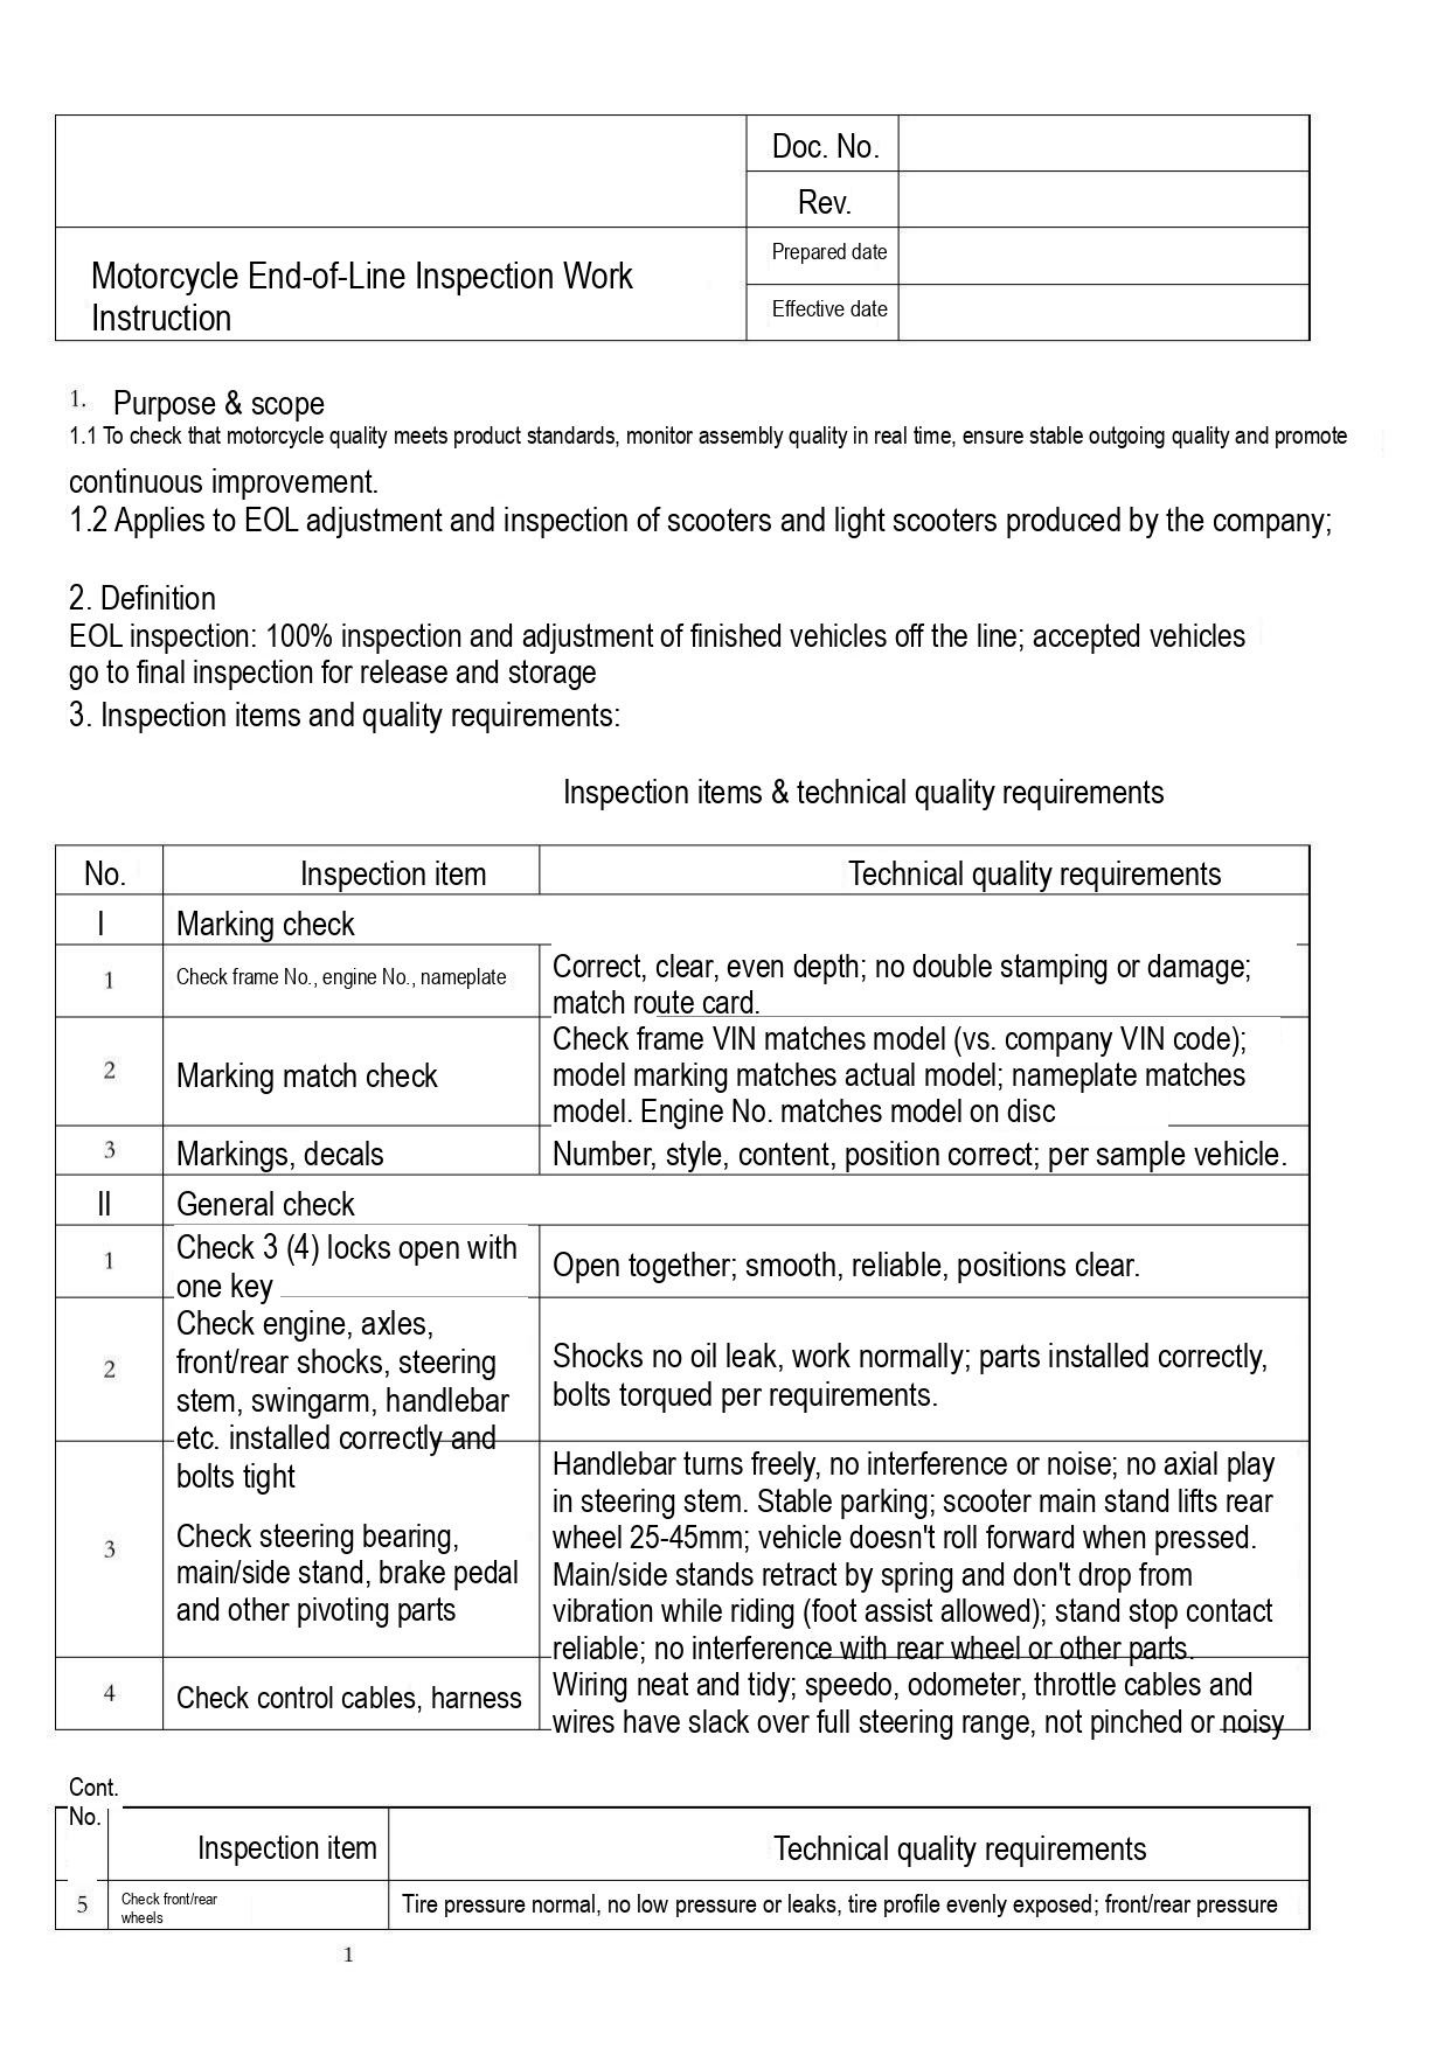| Motorcycle End-of-Line Inspection Work Instruction | Doc. No. | |
|---|---|---|
| | Rev. | |
| | Prepared date | |
| | Effective date | |

1. Purpose & scope
1.1 To check that motorcycle quality meets product standards, monitor assembly quality in real time, ensure stable outgoing quality and promote continuous improvement.
1.2 Applies to EOL adjustment and inspection of scooters and light scooters produced by the company;

2. Definition
EOL inspection: 100% inspection and adjustment of finished vehicles off the line; accepted vehicles go to final inspection for release and storage
3. Inspection items and quality requirements:

Inspection items & technical quality requirements

| No. | Inspection item | Technical quality requirements |
|---|---|---|
| I | Marking check | |
| 1 | Check frame No., engine No., nameplate | Correct, clear, even depth; no double stamping or damage; match route card. |
| 2 | Marking match check | Check frame VIN matches model (vs. company VIN code); model marking matches actual model; nameplate matches model. Engine No. matches model on disc |
| 3 | Markings, decals | Number, style, content, position correct; per sample vehicle. |
| II | General check | |
| 1 | Check 3 (4) locks open with one key | Open together; smooth, reliable, positions clear. |
| 2 | Check engine, axles, front/rear shocks, steering stem, swingarm, handlebar etc. installed correctly and bolts tight | Shocks no oil leak, work normally; parts installed correctly, bolts torqued per requirements. |
| 3 | Check steering bearing, main/side stand, brake pedal and other pivoting parts | Handlebar turns freely, no interference or noise; no axial play in steering stem. Stable parking; scooter main stand lifts rear wheel 25-45mm; vehicle doesn't roll forward when pressed. Main/side stands retract by spring and don't drop from vibration while riding (foot assist allowed); stand stop contact reliable; no interference with rear wheel or other parts. |
| 4 | Check control cables, harness | Wiring neat and tidy; speedo, odometer, throttle cables and wires have slack over full steering range, not pinched or noisy |

Cont.

| No. | Inspection item | Technical quality requirements |
|---|---|---|
| 5 | Check front/rear wheels | Tire pressure normal, no low pressure or leaks, tire profile evenly exposed; front/rear pressure |

1
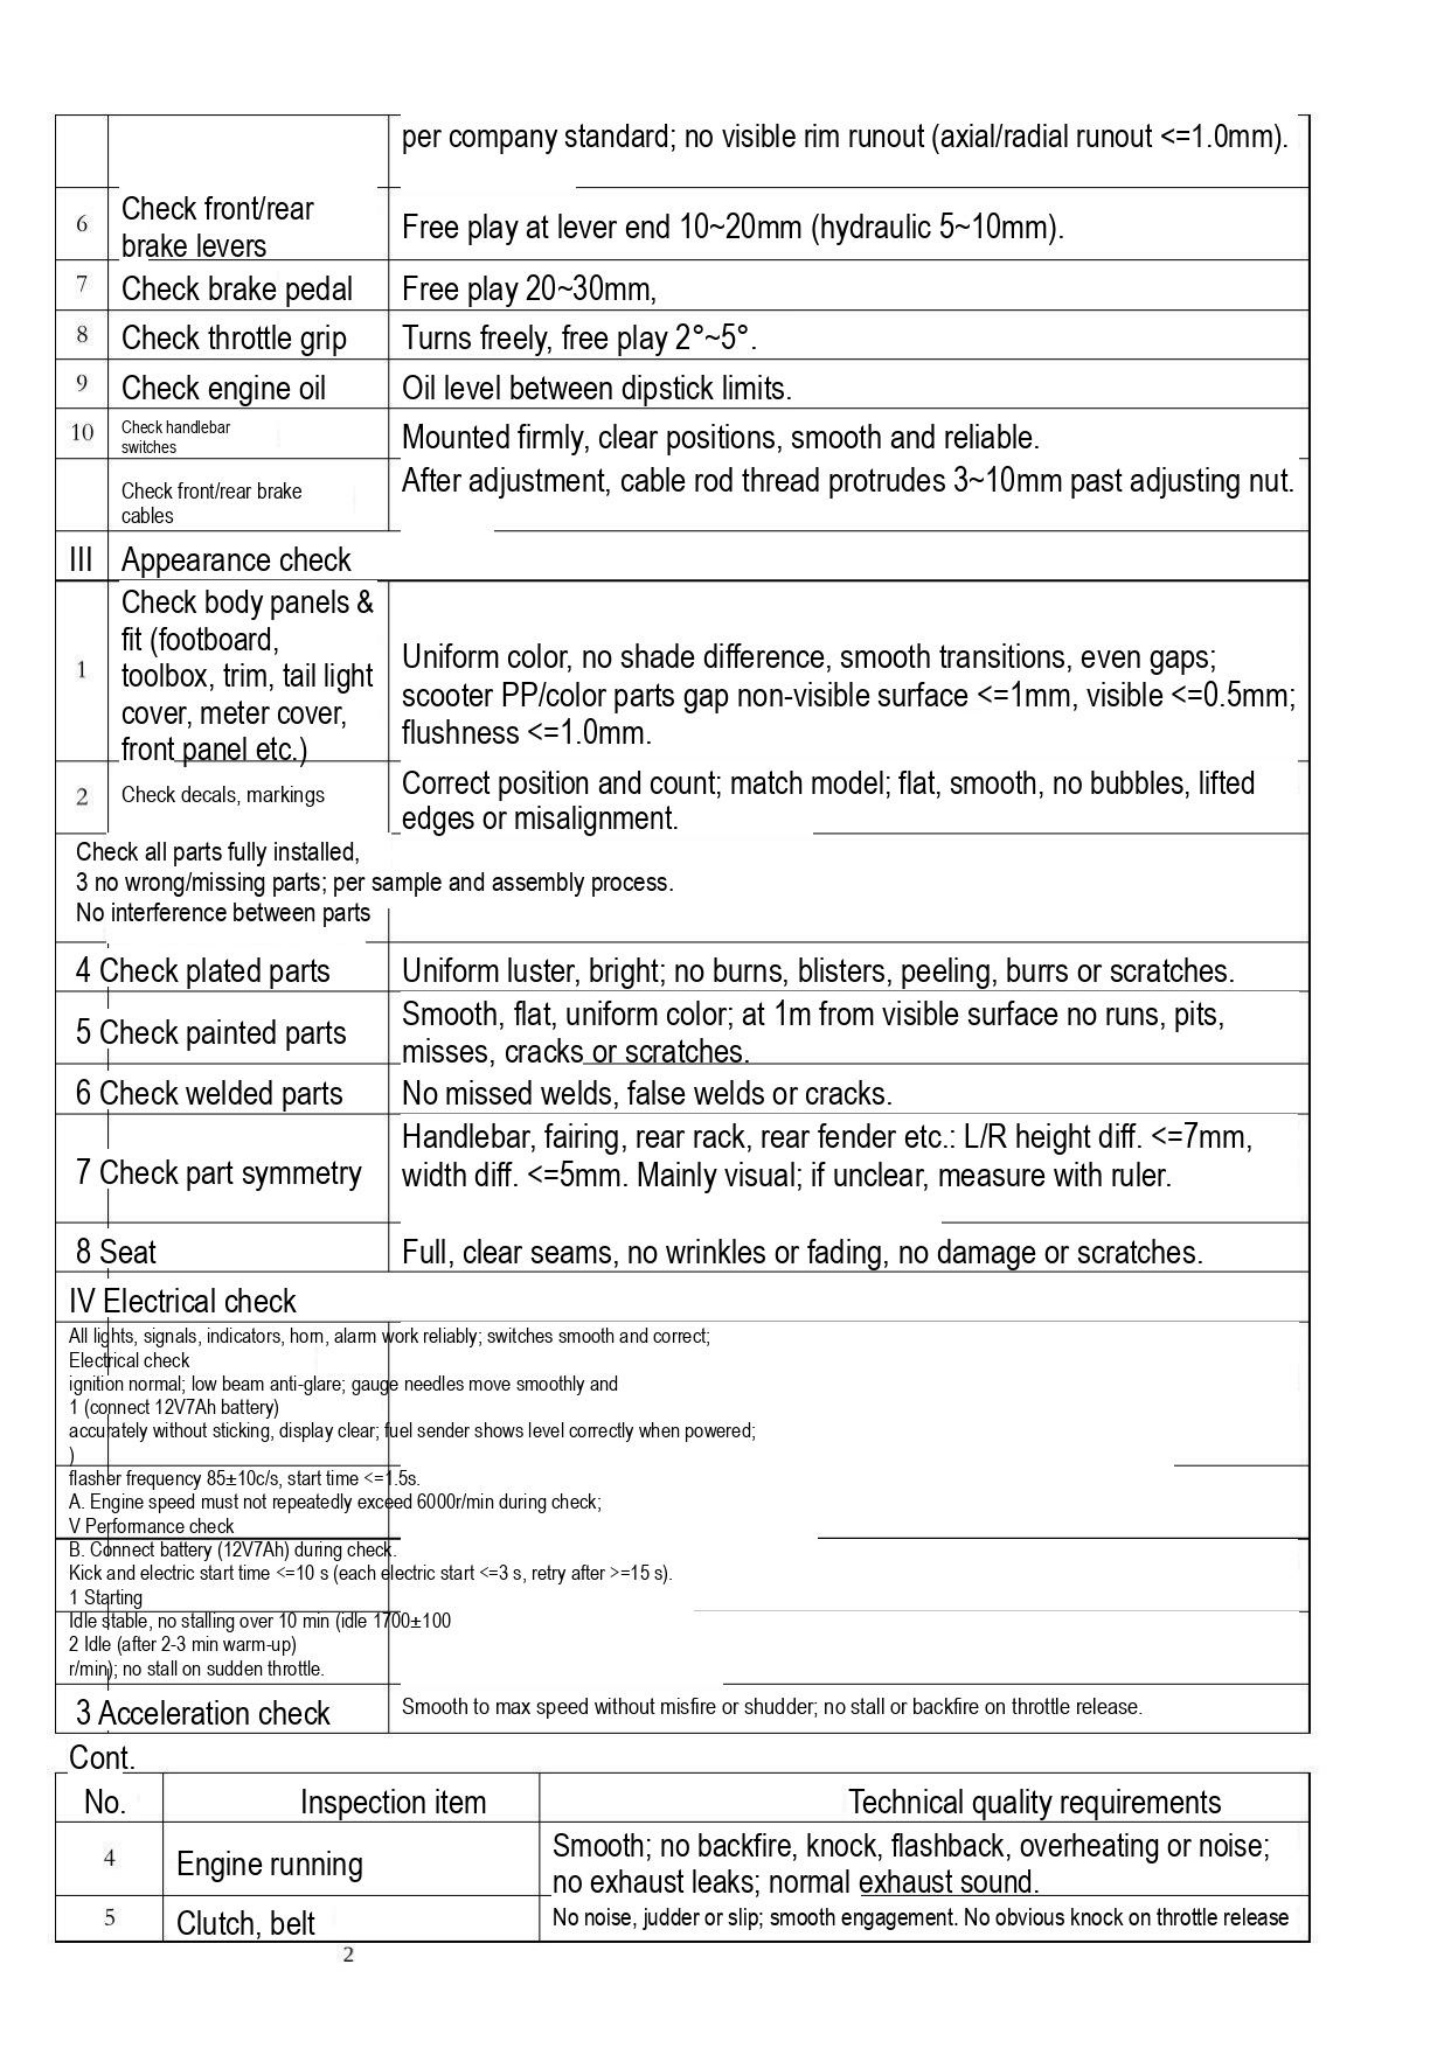| | | |
|---|---|---|
| | | per company standard; no visible rim runout (axial/radial runout <=1.0mm). |
| 6 | Check front/rear brake levers | Free play at lever end 10~20mm (hydraulic 5~10mm). |
| 7 | Check brake pedal | Free play 20~30mm, |
| 8 | Check throttle grip | Turns freely, free play 2°~5°. |
| 9 | Check engine oil | Oil level between dipstick limits. |
| 10 | Check handlebar switches | Mounted firmly, clear positions, smooth and reliable. |
| | Check front/rear brake cables | After adjustment, cable rod thread protrudes 3~10mm past adjusting nut. |
| III | Appearance check | |
| 1 | Check body panels & fit (footboard, toolbox, trim, tail light cover, meter cover, front panel etc.) | Uniform color, no shade difference, smooth transitions, even gaps; scooter PP/color parts gap non-visible surface <=1mm, visible <=0.5mm; flushness <=1.0mm. |
| 2 | Check decals, markings | Correct position and count; match model; flat, smooth, no bubbles, lifted edges or misalignment. |
| 3 | Check all parts fully installed, No interference between parts | no wrong/missing parts; per sample and assembly process. |
| 4 | Check plated parts | Uniform luster, bright; no burns, blisters, peeling, burrs or scratches. |
| 5 | Check painted parts | Smooth, flat, uniform color; at 1m from visible surface no runs, pits, misses, cracks or scratches. |
| 6 | Check welded parts | No missed welds, false welds or cracks. |
| 7 | Check part symmetry | Handlebar, fairing, rear rack, rear fender etc.: L/R height diff. <=7mm, width diff. <=5mm. Mainly visual; if unclear, measure with ruler. |
| 8 | Seat | Full, clear seams, no wrinkles or fading, no damage or scratches. |
| IV | Electrical check | |
| 1 | Electrical check (connect 12V7Ah battery) | All lights, signals, indicators, horn, alarm work reliably; switches smooth and correct; ignition normal; low beam anti-glare; gauge needles move smoothly and accurately without sticking, display clear; fuel sender shows level correctly when powered; flasher frequency 85±10c/s, start time <=1.5s. |
| V | Performance check | A. Engine speed must not repeatedly exceed 6000r/min during check; B. Connect battery (12V7Ah) during check. |
| 1 | Starting | Kick and electric start time <=10 s (each electric start <=3 s, retry after >=15 s). |
| 2 | Idle (after 2-3 min warm-up) | Idle stable, no stalling over 10 min (idle 1700±100 r/min); no stall on sudden throttle. |
| 3 | Acceleration check | Smooth to max speed without misfire or shudder; no stall or backfire on throttle release. |

Cont.

| No. | Inspection item | Technical quality requirements |
|---|---|---|
| 4 | Engine running | Smooth; no backfire, knock, flashback, overheating or noise; no exhaust leaks; normal exhaust sound. |
| 5 | Clutch, belt | No noise, judder or slip; smooth engagement. No obvious knock on throttle release |

2
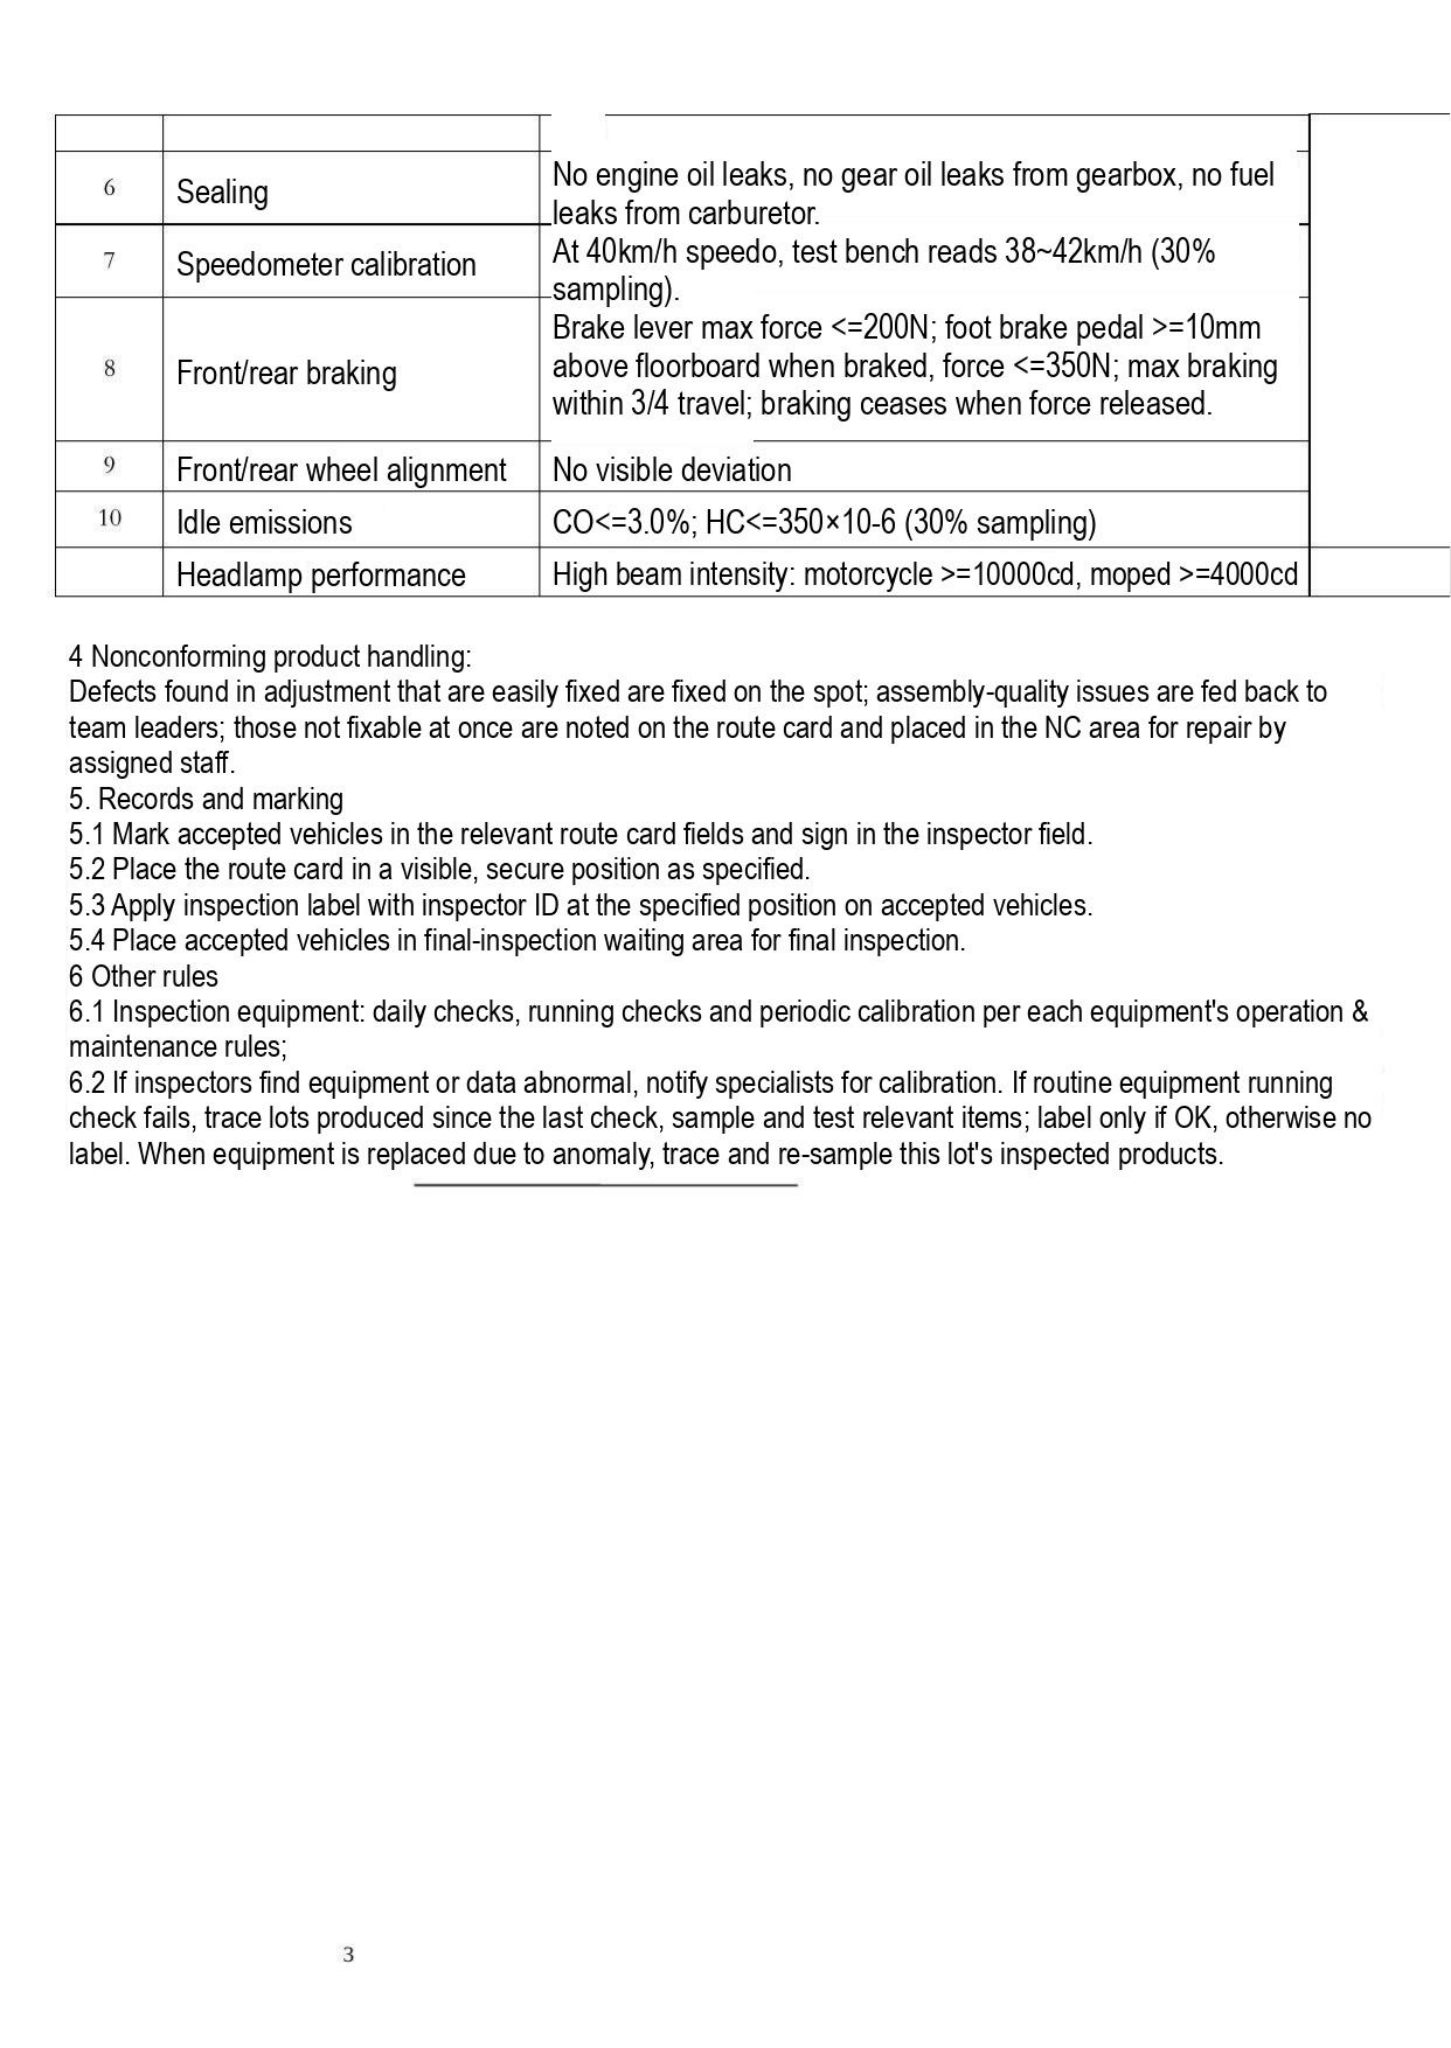| | | | |
|---|---|---|---|
| 6 | Sealing | No engine oil leaks, no gear oil leaks from gearbox, no fuel leaks from carburetor. | |
| 7 | Speedometer calibration | At 40km/h speedo, test bench reads 38~42km/h (30% sampling). | |
| 8 | Front/rear braking | Brake lever max force <=200N; foot brake pedal >=10mm above floorboard when braked, force <=350N; max braking within 3/4 travel; braking ceases when force released. | |
| 9 | Front/rear wheel alignment | No visible deviation | |
| 10 | Idle emissions | CO<=3.0%; HC<=350×10-6 (30% sampling) | |
| | Headlamp performance | High beam intensity: motorcycle >=10000cd, moped >=4000cd | |

4 Nonconforming product handling:
Defects found in adjustment that are easily fixed are fixed on the spot; assembly-quality issues are fed back to team leaders; those not fixable at once are noted on the route card and placed in the NC area for repair by assigned staff.
5. Records and marking
5.1 Mark accepted vehicles in the relevant route card fields and sign in the inspector field.
5.2 Place the route card in a visible, secure position as specified.
5.3 Apply inspection label with inspector ID at the specified position on accepted vehicles.
5.4 Place accepted vehicles in final-inspection waiting area for final inspection.
6 Other rules
6.1 Inspection equipment: daily checks, running checks and periodic calibration per each equipment's operation & maintenance rules;
6.2 If inspectors find equipment or data abnormal, notify specialists for calibration. If routine equipment running check fails, trace lots produced since the last check, sample and test relevant items; label only if OK, otherwise no label. When equipment is replaced due to anomaly, trace and re-sample this lot's inspected products.

3